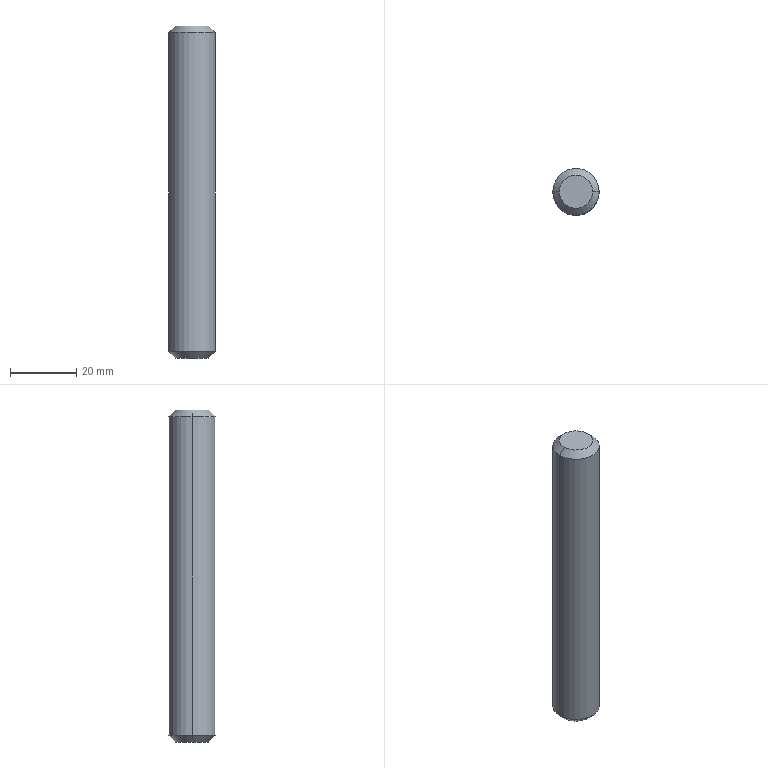Part | STEP file | CHOT 14X100 | 1 solid | 8 faces | box 14 x 14 x 100 mm | volume 15235 mm3 | cone 4 | cylinder 2 | plane 2 | commonest cylinder face diameters 14 x2
STEP:
#1=CARTESIAN_POINT('',(0.,0.,0.));
#2=DIRECTION('',(0.,0.,1.));
#3=DIRECTION('',(1.,0.,0.));
#4=AXIS2_PLACEMENT_3D('',#1,#2,#3);
#5=CARTESIAN_POINT('',(7.,0.,2.));
#6=VERTEX_POINT('',#5);
#7=CARTESIAN_POINT('',(-7.,0.,2.));
#8=VERTEX_POINT('',#7);
#9=CARTESIAN_POINT('',(0.,0.,2.));
#10=DIRECTION('',(0.,0.,1.));
#11=DIRECTION('',(1.,0.,0.));
#12=AXIS2_PLACEMENT_3D('',#9,#10,#11);
#13=CIRCLE('',#12,7.);
#14=CARTESIAN_POINT('',(0.,0.,0.));
#15=DIRECTION('',(0.,0.,1.));
#16=DIRECTION('',(1.,0.,0.));
#17=AXIS2_PLACEMENT_3D('',#14,#15,#16);
#18=CYLINDRICAL_SURFACE('',#17,7.);
#19=CARTESIAN_POINT('',(0.,2.));
#20=DIRECTION('',(1.,0.));
#21=VECTOR('',#20,1.);
#22=LINE('',#19,#21);
#23=(GEOMETRIC_REPRESENTATION_CONTEXT(2)PARAMETRIC_REPRESENTATION_CONTEXT()REPRESENTATION_CONTEXT('',''));
#24=DEFINITIONAL_REPRESENTATION('',(#22),#23);
#25=PCURVE('',#18,#24);
#26=CARTESIAN_POINT('',(0.,0.,2.));
#27=DIRECTION('',(0.,0.,1.));
#28=DIRECTION('',(1.,0.,0.));
#29=AXIS2_PLACEMENT_3D('',#26,#27,#28);
#30=CONICAL_SURFACE('',#29,7.,0.7854);
#31=CARTESIAN_POINT('',(0.,0.));
#32=DIRECTION('',(1.,0.));
#33=VECTOR('',#32,1.);
#34=LINE('',#31,#33);
#35=(GEOMETRIC_REPRESENTATION_CONTEXT(2)PARAMETRIC_REPRESENTATION_CONTEXT()REPRESENTATION_CONTEXT('',''));
#36=DEFINITIONAL_REPRESENTATION('',(#34),#35);
#37=PCURVE('',#30,#36);
#38=SURFACE_CURVE('',#13,(#25,#37),.PCURVE_S1.);
#39=EDGE_CURVE('',#6,#8,#38,.T.);
#40=ORIENTED_EDGE('',*,*,#39,.T.);
#41=CARTESIAN_POINT('',(-7.,0.,98.));
#42=VERTEX_POINT('',#41);
#43=CARTESIAN_POINT('',(-7.,0.,0.));
#44=DIRECTION('',(0.,0.,1.));
#45=VECTOR('',#44,1.);
#46=LINE('',#43,#45);
#47=CARTESIAN_POINT('',(3.142,0.));
#48=DIRECTION('',(0.,1.));
#49=VECTOR('',#48,1.);
#50=LINE('',#47,#49);
#51=(GEOMETRIC_REPRESENTATION_CONTEXT(2)PARAMETRIC_REPRESENTATION_CONTEXT()REPRESENTATION_CONTEXT('',''));
#52=DEFINITIONAL_REPRESENTATION('',(#50),#51);
#53=PCURVE('',#18,#52);
#54=CARTESIAN_POINT('',(0.,0.,0.));
#55=DIRECTION('',(0.,0.,1.));
#56=DIRECTION('',(1.,0.,0.));
#57=AXIS2_PLACEMENT_3D('',#54,#55,#56);
#58=CYLINDRICAL_SURFACE('',#57,7.);
#59=CARTESIAN_POINT('',(3.142,0.));
#60=DIRECTION('',(0.,1.));
#61=VECTOR('',#60,1.);
#62=LINE('',#59,#61);
#63=(GEOMETRIC_REPRESENTATION_CONTEXT(2)PARAMETRIC_REPRESENTATION_CONTEXT()REPRESENTATION_CONTEXT('',''));
#64=DEFINITIONAL_REPRESENTATION('',(#62),#63);
#65=PCURVE('',#58,#64);
#66=SURFACE_CURVE('',#46,(#53,#65),.PCURVE_S1.);
#67=EDGE_CURVE('',#8,#42,#66,.T.);
#68=ORIENTED_EDGE('',*,*,#67,.T.);
#69=CARTESIAN_POINT('',(7.,0.,98.));
#70=VERTEX_POINT('',#69);
#71=CARTESIAN_POINT('',(0.,0.,98.));
#72=DIRECTION('',(0.,0.,-1.));
#73=DIRECTION('',(1.,0.,0.));
#74=AXIS2_PLACEMENT_3D('',#71,#72,#73);
#75=CIRCLE('',#74,7.);
#76=CARTESIAN_POINT('',(6.283,98.));
#77=DIRECTION('',(-1.,0.));
#78=VECTOR('',#77,1.);
#79=LINE('',#76,#78);
#80=(GEOMETRIC_REPRESENTATION_CONTEXT(2)PARAMETRIC_REPRESENTATION_CONTEXT()REPRESENTATION_CONTEXT('',''));
#81=DEFINITIONAL_REPRESENTATION('',(#79),#80);
#82=PCURVE('',#18,#81);
#83=CARTESIAN_POINT('',(0.,0.,98.));
#84=DIRECTION('',(0.,0.,-1.));
#85=DIRECTION('',(-1.,0.,0.));
#86=AXIS2_PLACEMENT_3D('',#83,#84,#85);
#87=CONICAL_SURFACE('',#86,7.,0.7854);
#88=CARTESIAN_POINT('',(-3.142,0.));
#89=DIRECTION('',(1.,0.));
#90=VECTOR('',#89,1.);
#91=LINE('',#88,#90);
#92=(GEOMETRIC_REPRESENTATION_CONTEXT(2)PARAMETRIC_REPRESENTATION_CONTEXT()REPRESENTATION_CONTEXT('',''));
#93=DEFINITIONAL_REPRESENTATION('',(#91),#92);
#94=PCURVE('',#87,#93);
#95=SURFACE_CURVE('',#75,(#82,#94),.PCURVE_S1.);
#96=EDGE_CURVE('',#42,#70,#95,.T.);
#97=ORIENTED_EDGE('',*,*,#96,.T.);
#98=CARTESIAN_POINT('',(7.,0.,0.));
#99=DIRECTION('',(0.,0.,1.));
#100=VECTOR('',#99,1.);
#101=LINE('',#98,#100);
#102=CARTESIAN_POINT('',(0.,0.));
#103=DIRECTION('',(0.,1.));
#104=VECTOR('',#103,1.);
#105=LINE('',#102,#104);
#106=(GEOMETRIC_REPRESENTATION_CONTEXT(2)PARAMETRIC_REPRESENTATION_CONTEXT()REPRESENTATION_CONTEXT('',''));
#107=DEFINITIONAL_REPRESENTATION('',(#105),#106);
#108=PCURVE('',#18,#107);
#109=CARTESIAN_POINT('',(6.283,0.));
#110=DIRECTION('',(0.,1.));
#111=VECTOR('',#110,1.);
#112=LINE('',#109,#111);
#113=(GEOMETRIC_REPRESENTATION_CONTEXT(2)PARAMETRIC_REPRESENTATION_CONTEXT()REPRESENTATION_CONTEXT('',''));
#114=DEFINITIONAL_REPRESENTATION('',(#112),#113);
#115=PCURVE('',#58,#114);
#116=SURFACE_CURVE('',#101,(#108,#115),.PCURVE_S1.);
#117=EDGE_CURVE('',#6,#70,#116,.T.);
#118=ORIENTED_EDGE('',*,*,#117,.F.);
#119=EDGE_LOOP('',(#40,#68,#97,#118));
#120=FACE_BOUND('',#119,.T.);
#121=ADVANCED_FACE('',(#120),#18,.T.);
#122=CARTESIAN_POINT('',(5.,0.,-0.000000001));
#123=VERTEX_POINT('',#122);
#124=CARTESIAN_POINT('',(-5.,0.,-0.000000001));
#125=VERTEX_POINT('',#124);
#126=CARTESIAN_POINT('',(0.,0.,-0.000000001));
#127=DIRECTION('',(0.,0.,1.));
#128=DIRECTION('',(1.,0.,0.));
#129=AXIS2_PLACEMENT_3D('',#126,#127,#128);
#130=CIRCLE('',#129,5.);
#131=CARTESIAN_POINT('',(0.,-2.));
#132=DIRECTION('',(1.,0.));
#133=VECTOR('',#132,1.);
#134=LINE('',#131,#133);
#135=(GEOMETRIC_REPRESENTATION_CONTEXT(2)PARAMETRIC_REPRESENTATION_CONTEXT()REPRESENTATION_CONTEXT('',''));
#136=DEFINITIONAL_REPRESENTATION('',(#134),#135);
#137=PCURVE('',#30,#136);
#138=CARTESIAN_POINT('',(0.,0.,0.));
#139=DIRECTION('',(0.,0.,-1.));
#140=DIRECTION('',(-1.,0.,0.));
#141=AXIS2_PLACEMENT_3D('',#138,#139,#140);
#142=PLANE('',#141);
#143=CARTESIAN_POINT('',(-5.,0.));
#144=CARTESIAN_POINT('',(-5.,8.66));
#145=CARTESIAN_POINT('',(2.5,4.33));
#146=CARTESIAN_POINT('',(10.,0.));
#147=CARTESIAN_POINT('',(2.5,-4.33));
#148=CARTESIAN_POINT('',(-5.,-8.66));
#149=CARTESIAN_POINT('',(-5.,0.));
#150=(BOUNDED_CURVE()B_SPLINE_CURVE(2,(#143,#144,#145,#146,#147,#148,#149),.UNSPECIFIED.,.T.,.F.)B_SPLINE_CURVE_WITH_KNOTS((1,2,2,2,2,1),(-2.094,0.,2.094,4.189,6.283,8.378),.UNSPECIFIED.)CURVE()GEOMETRIC_REPRESENTATION_ITEM()RATIONAL_B_SPLINE_CURVE((1.,0.5,1.,0.5,1.,0.5,1.))REPRESENTATION_ITEM(''));
#151=(GEOMETRIC_REPRESENTATION_CONTEXT(2)PARAMETRIC_REPRESENTATION_CONTEXT()REPRESENTATION_CONTEXT('',''));
#152=DEFINITIONAL_REPRESENTATION('',(#150),#151);
#153=PCURVE('',#142,#152);
#154=SURFACE_CURVE('',#130,(#137,#153),.PCURVE_S1.);
#155=EDGE_CURVE('',#123,#125,#154,.T.);
#156=ORIENTED_EDGE('',*,*,#155,.T.);
#157=CARTESIAN_POINT('',(-7.,0.,2.));
#158=DIRECTION('',(-0.7071,0.,0.7071));
#159=VECTOR('',#158,1.);
#160=LINE('',#157,#159);
#161=CARTESIAN_POINT('',(3.142,0.));
#162=DIRECTION('',(0.,1.));
#163=VECTOR('',#162,1.);
#164=LINE('',#161,#163);
#165=(GEOMETRIC_REPRESENTATION_CONTEXT(2)PARAMETRIC_REPRESENTATION_CONTEXT()REPRESENTATION_CONTEXT('',''));
#166=DEFINITIONAL_REPRESENTATION('',(#164),#165);
#167=PCURVE('',#30,#166);
#168=CARTESIAN_POINT('',(0.,0.,2.));
#169=DIRECTION('',(0.,0.,1.));
#170=DIRECTION('',(1.,0.,0.));
#171=AXIS2_PLACEMENT_3D('',#168,#169,#170);
#172=CONICAL_SURFACE('',#171,7.,0.7854);
#173=CARTESIAN_POINT('',(3.142,0.));
#174=DIRECTION('',(0.,1.));
#175=VECTOR('',#174,1.);
#176=LINE('',#173,#175);
#177=(GEOMETRIC_REPRESENTATION_CONTEXT(2)PARAMETRIC_REPRESENTATION_CONTEXT()REPRESENTATION_CONTEXT('',''));
#178=DEFINITIONAL_REPRESENTATION('',(#176),#177);
#179=PCURVE('',#172,#178);
#180=SURFACE_CURVE('',#160,(#167,#179),.PCURVE_S1.);
#181=EDGE_CURVE('',#125,#8,#180,.T.);
#182=ORIENTED_EDGE('',*,*,#181,.T.);
#183=ORIENTED_EDGE('',*,*,#39,.F.);
#184=CARTESIAN_POINT('',(7.,0.,2.));
#185=DIRECTION('',(0.7071,0.,0.7071));
#186=VECTOR('',#185,1.);
#187=LINE('',#184,#186);
#188=CARTESIAN_POINT('',(0.,0.));
#189=DIRECTION('',(0.,1.));
#190=VECTOR('',#189,1.);
#191=LINE('',#188,#190);
#192=(GEOMETRIC_REPRESENTATION_CONTEXT(2)PARAMETRIC_REPRESENTATION_CONTEXT()REPRESENTATION_CONTEXT('',''));
#193=DEFINITIONAL_REPRESENTATION('',(#191),#192);
#194=PCURVE('',#30,#193);
#195=CARTESIAN_POINT('',(6.283,0.));
#196=DIRECTION('',(0.,1.));
#197=VECTOR('',#196,1.);
#198=LINE('',#195,#197);
#199=(GEOMETRIC_REPRESENTATION_CONTEXT(2)PARAMETRIC_REPRESENTATION_CONTEXT()REPRESENTATION_CONTEXT('',''));
#200=DEFINITIONAL_REPRESENTATION('',(#198),#199);
#201=PCURVE('',#172,#200);
#202=SURFACE_CURVE('',#187,(#194,#201),.PCURVE_S1.);
#203=EDGE_CURVE('',#123,#6,#202,.T.);
#204=ORIENTED_EDGE('',*,*,#203,.F.);
#205=EDGE_LOOP('',(#156,#182,#183,#204));
#206=FACE_BOUND('',#205,.T.);
#207=ADVANCED_FACE('',(#206),#30,.T.);
#208=CARTESIAN_POINT('',(-5.,0.,100.));
#209=VERTEX_POINT('',#208);
#210=CARTESIAN_POINT('',(5.,0.,100.));
#211=VERTEX_POINT('',#210);
#212=CARTESIAN_POINT('',(0.,0.,100.));
#213=DIRECTION('',(0.,0.,-1.));
#214=DIRECTION('',(-1.,0.,0.));
#215=AXIS2_PLACEMENT_3D('',#212,#213,#214);
#216=CIRCLE('',#215,5.);
#217=CARTESIAN_POINT('',(0.,-2.));
#218=DIRECTION('',(1.,0.));
#219=VECTOR('',#218,1.);
#220=LINE('',#217,#219);
#221=(GEOMETRIC_REPRESENTATION_CONTEXT(2)PARAMETRIC_REPRESENTATION_CONTEXT()REPRESENTATION_CONTEXT('',''));
#222=DEFINITIONAL_REPRESENTATION('',(#220),#221);
#223=PCURVE('',#87,#222);
#224=CARTESIAN_POINT('',(0.,0.,100.));
#225=DIRECTION('',(0.,0.,-1.));
#226=DIRECTION('',(-1.,0.,0.));
#227=AXIS2_PLACEMENT_3D('',#224,#225,#226);
#228=PLANE('',#227);
#229=CARTESIAN_POINT('',(0.,0.));
#230=DIRECTION('',(1.,0.));
#231=AXIS2_PLACEMENT_2D('',#229,#230);
#232=CIRCLE('',#231,5.);
#233=(GEOMETRIC_REPRESENTATION_CONTEXT(2)PARAMETRIC_REPRESENTATION_CONTEXT()REPRESENTATION_CONTEXT('',''));
#234=DEFINITIONAL_REPRESENTATION('',(#232),#233);
#235=PCURVE('',#228,#234);
#236=SURFACE_CURVE('',#216,(#223,#235),.PCURVE_S1.);
#237=EDGE_CURVE('',#209,#211,#236,.T.);
#238=ORIENTED_EDGE('',*,*,#237,.T.);
#239=CARTESIAN_POINT('',(7.,0.,98.));
#240=DIRECTION('',(0.7071,0.,-0.7071));
#241=VECTOR('',#240,1.);
#242=LINE('',#239,#241);
#243=CARTESIAN_POINT('',(3.142,0.));
#244=DIRECTION('',(0.,1.));
#245=VECTOR('',#244,1.);
#246=LINE('',#243,#245);
#247=(GEOMETRIC_REPRESENTATION_CONTEXT(2)PARAMETRIC_REPRESENTATION_CONTEXT()REPRESENTATION_CONTEXT('',''));
#248=DEFINITIONAL_REPRESENTATION('',(#246),#247);
#249=PCURVE('',#87,#248);
#250=CARTESIAN_POINT('',(0.,0.,98.));
#251=DIRECTION('',(0.,0.,-1.));
#252=DIRECTION('',(-1.,0.,0.));
#253=AXIS2_PLACEMENT_3D('',#250,#251,#252);
#254=CONICAL_SURFACE('',#253,7.,0.7854);
#255=CARTESIAN_POINT('',(3.142,0.));
#256=DIRECTION('',(0.,1.));
#257=VECTOR('',#256,1.);
#258=LINE('',#255,#257);
#259=(GEOMETRIC_REPRESENTATION_CONTEXT(2)PARAMETRIC_REPRESENTATION_CONTEXT()REPRESENTATION_CONTEXT('',''));
#260=DEFINITIONAL_REPRESENTATION('',(#258),#259);
#261=PCURVE('',#254,#260);
#262=SURFACE_CURVE('',#242,(#249,#261),.PCURVE_S1.);
#263=EDGE_CURVE('',#211,#70,#262,.T.);
#264=ORIENTED_EDGE('',*,*,#263,.T.);
#265=ORIENTED_EDGE('',*,*,#96,.F.);
#266=CARTESIAN_POINT('',(-7.,0.,98.));
#267=DIRECTION('',(-0.7071,0.,-0.7071));
#268=VECTOR('',#267,1.);
#269=LINE('',#266,#268);
#270=CARTESIAN_POINT('',(0.,0.));
#271=DIRECTION('',(0.,1.));
#272=VECTOR('',#271,1.);
#273=LINE('',#270,#272);
#274=(GEOMETRIC_REPRESENTATION_CONTEXT(2)PARAMETRIC_REPRESENTATION_CONTEXT()REPRESENTATION_CONTEXT('',''));
#275=DEFINITIONAL_REPRESENTATION('',(#273),#274);
#276=PCURVE('',#87,#275);
#277=CARTESIAN_POINT('',(6.283,0.));
#278=DIRECTION('',(0.,1.));
#279=VECTOR('',#278,1.);
#280=LINE('',#277,#279);
#281=(GEOMETRIC_REPRESENTATION_CONTEXT(2)PARAMETRIC_REPRESENTATION_CONTEXT()REPRESENTATION_CONTEXT('',''));
#282=DEFINITIONAL_REPRESENTATION('',(#280),#281);
#283=PCURVE('',#254,#282);
#284=SURFACE_CURVE('',#269,(#276,#283),.PCURVE_S1.);
#285=EDGE_CURVE('',#209,#42,#284,.T.);
#286=ORIENTED_EDGE('',*,*,#285,.F.);
#287=EDGE_LOOP('',(#238,#264,#265,#286));
#288=FACE_BOUND('',#287,.T.);
#289=ADVANCED_FACE('',(#288),#87,.T.);
#290=ORIENTED_EDGE('',*,*,#67,.F.);
#291=CARTESIAN_POINT('',(0.,0.,2.));
#292=DIRECTION('',(0.,0.,1.));
#293=DIRECTION('',(1.,0.,0.));
#294=AXIS2_PLACEMENT_3D('',#291,#292,#293);
#295=CIRCLE('',#294,7.);
#296=CARTESIAN_POINT('',(0.,2.));
#297=DIRECTION('',(1.,0.));
#298=VECTOR('',#297,1.);
#299=LINE('',#296,#298);
#300=(GEOMETRIC_REPRESENTATION_CONTEXT(2)PARAMETRIC_REPRESENTATION_CONTEXT()REPRESENTATION_CONTEXT('',''));
#301=DEFINITIONAL_REPRESENTATION('',(#299),#300);
#302=PCURVE('',#58,#301);
#303=CARTESIAN_POINT('',(0.,0.));
#304=DIRECTION('',(1.,0.));
#305=VECTOR('',#304,1.);
#306=LINE('',#303,#305);
#307=(GEOMETRIC_REPRESENTATION_CONTEXT(2)PARAMETRIC_REPRESENTATION_CONTEXT()REPRESENTATION_CONTEXT('',''));
#308=DEFINITIONAL_REPRESENTATION('',(#306),#307);
#309=PCURVE('',#172,#308);
#310=SURFACE_CURVE('',#295,(#302,#309),.PCURVE_S1.);
#311=EDGE_CURVE('',#8,#6,#310,.T.);
#312=ORIENTED_EDGE('',*,*,#311,.T.);
#313=ORIENTED_EDGE('',*,*,#117,.T.);
#314=CARTESIAN_POINT('',(0.,0.,98.));
#315=DIRECTION('',(0.,0.,-1.));
#316=DIRECTION('',(1.,0.,0.));
#317=AXIS2_PLACEMENT_3D('',#314,#315,#316);
#318=CIRCLE('',#317,7.);
#319=CARTESIAN_POINT('',(6.283,98.));
#320=DIRECTION('',(-1.,0.));
#321=VECTOR('',#320,1.);
#322=LINE('',#319,#321);
#323=(GEOMETRIC_REPRESENTATION_CONTEXT(2)PARAMETRIC_REPRESENTATION_CONTEXT()REPRESENTATION_CONTEXT('',''));
#324=DEFINITIONAL_REPRESENTATION('',(#322),#323);
#325=PCURVE('',#58,#324);
#326=CARTESIAN_POINT('',(3.142,0.));
#327=DIRECTION('',(1.,0.));
#328=VECTOR('',#327,1.);
#329=LINE('',#326,#328);
#330=(GEOMETRIC_REPRESENTATION_CONTEXT(2)PARAMETRIC_REPRESENTATION_CONTEXT()REPRESENTATION_CONTEXT('',''));
#331=DEFINITIONAL_REPRESENTATION('',(#329),#330);
#332=PCURVE('',#254,#331);
#333=SURFACE_CURVE('',#318,(#325,#332),.PCURVE_S1.);
#334=EDGE_CURVE('',#70,#42,#333,.T.);
#335=ORIENTED_EDGE('',*,*,#334,.T.);
#336=EDGE_LOOP('',(#290,#312,#313,#335));
#337=FACE_BOUND('',#336,.T.);
#338=ADVANCED_FACE('',(#337),#58,.T.);
#339=ORIENTED_EDGE('',*,*,#181,.F.);
#340=CARTESIAN_POINT('',(0.,0.,-0.000000001));
#341=DIRECTION('',(0.,0.,1.));
#342=DIRECTION('',(1.,0.,0.));
#343=AXIS2_PLACEMENT_3D('',#340,#341,#342);
#344=CIRCLE('',#343,5.);
#345=CARTESIAN_POINT('',(0.,-2.));
#346=DIRECTION('',(1.,0.));
#347=VECTOR('',#346,1.);
#348=LINE('',#345,#347);
#349=(GEOMETRIC_REPRESENTATION_CONTEXT(2)PARAMETRIC_REPRESENTATION_CONTEXT()REPRESENTATION_CONTEXT('',''));
#350=DEFINITIONAL_REPRESENTATION('',(#348),#349);
#351=PCURVE('',#172,#350);
#352=CARTESIAN_POINT('',(-5.,0.));
#353=CARTESIAN_POINT('',(-5.,8.66));
#354=CARTESIAN_POINT('',(2.5,4.33));
#355=CARTESIAN_POINT('',(10.,0.));
#356=CARTESIAN_POINT('',(2.5,-4.33));
#357=CARTESIAN_POINT('',(-5.,-8.66));
#358=CARTESIAN_POINT('',(-5.,0.));
#359=(BOUNDED_CURVE()B_SPLINE_CURVE(2,(#352,#353,#354,#355,#356,#357,#358),.UNSPECIFIED.,.T.,.F.)B_SPLINE_CURVE_WITH_KNOTS((1,2,2,2,2,1),(-2.094,0.,2.094,4.189,6.283,8.378),.UNSPECIFIED.)CURVE()GEOMETRIC_REPRESENTATION_ITEM()RATIONAL_B_SPLINE_CURVE((1.,0.5,1.,0.5,1.,0.5,1.))REPRESENTATION_ITEM(''));
#360=(GEOMETRIC_REPRESENTATION_CONTEXT(2)PARAMETRIC_REPRESENTATION_CONTEXT()REPRESENTATION_CONTEXT('',''));
#361=DEFINITIONAL_REPRESENTATION('',(#359),#360);
#362=PCURVE('',#142,#361);
#363=SURFACE_CURVE('',#344,(#351,#362),.PCURVE_S1.);
#364=EDGE_CURVE('',#125,#123,#363,.T.);
#365=ORIENTED_EDGE('',*,*,#364,.T.);
#366=ORIENTED_EDGE('',*,*,#203,.T.);
#367=ORIENTED_EDGE('',*,*,#311,.F.);
#368=EDGE_LOOP('',(#339,#365,#366,#367));
#369=FACE_BOUND('',#368,.T.);
#370=ADVANCED_FACE('',(#369),#172,.T.);
#371=ORIENTED_EDGE('',*,*,#263,.F.);
#372=CARTESIAN_POINT('',(0.,0.,100.));
#373=DIRECTION('',(0.,0.,-1.));
#374=DIRECTION('',(-1.,0.,0.));
#375=AXIS2_PLACEMENT_3D('',#372,#373,#374);
#376=CIRCLE('',#375,5.);
#377=CARTESIAN_POINT('',(0.,-2.));
#378=DIRECTION('',(1.,0.));
#379=VECTOR('',#378,1.);
#380=LINE('',#377,#379);
#381=(GEOMETRIC_REPRESENTATION_CONTEXT(2)PARAMETRIC_REPRESENTATION_CONTEXT()REPRESENTATION_CONTEXT('',''));
#382=DEFINITIONAL_REPRESENTATION('',(#380),#381);
#383=PCURVE('',#254,#382);
#384=CARTESIAN_POINT('',(0.,0.));
#385=DIRECTION('',(1.,0.));
#386=AXIS2_PLACEMENT_2D('',#384,#385);
#387=CIRCLE('',#386,5.);
#388=(GEOMETRIC_REPRESENTATION_CONTEXT(2)PARAMETRIC_REPRESENTATION_CONTEXT()REPRESENTATION_CONTEXT('',''));
#389=DEFINITIONAL_REPRESENTATION('',(#387),#388);
#390=PCURVE('',#228,#389);
#391=SURFACE_CURVE('',#376,(#383,#390),.PCURVE_S1.);
#392=EDGE_CURVE('',#211,#209,#391,.T.);
#393=ORIENTED_EDGE('',*,*,#392,.T.);
#394=ORIENTED_EDGE('',*,*,#285,.T.);
#395=ORIENTED_EDGE('',*,*,#334,.F.);
#396=EDGE_LOOP('',(#371,#393,#394,#395));
#397=FACE_BOUND('',#396,.T.);
#398=ADVANCED_FACE('',(#397),#254,.T.);
#399=ORIENTED_EDGE('',*,*,#155,.F.);
#400=ORIENTED_EDGE('',*,*,#364,.F.);
#401=EDGE_LOOP('',(#399,#400));
#402=FACE_BOUND('',#401,.T.);
#403=ADVANCED_FACE('',(#402),#142,.T.);
#404=ORIENTED_EDGE('',*,*,#237,.F.);
#405=ORIENTED_EDGE('',*,*,#392,.F.);
#406=EDGE_LOOP('',(#404,#405));
#407=FACE_BOUND('',#406,.T.);
#408=ADVANCED_FACE('',(#407),#228,.F.);
#409=CLOSED_SHELL('',(#121,#207,#289,#338,#370,#398,#403,#408));
#410=MANIFOLD_SOLID_BREP('',#409);
#411=(LENGTH_UNIT()NAMED_UNIT(*)SI_UNIT(.MILLI.,.METRE.));
#412=UNCERTAINTY_MEASURE_WITH_UNIT(LENGTH_MEASURE(0.0000001),#411,'','');
#413=(NAMED_UNIT(*)PLANE_ANGLE_UNIT()SI_UNIT($,.RADIAN.));
#414=(NAMED_UNIT(*)SI_UNIT($,.STERADIAN.)SOLID_ANGLE_UNIT());
#415=(GEOMETRIC_REPRESENTATION_CONTEXT(3)GLOBAL_UNCERTAINTY_ASSIGNED_CONTEXT((#412))GLOBAL_UNIT_ASSIGNED_CONTEXT((#411,#413,#414))REPRESENTATION_CONTEXT('',''));
#416=ADVANCED_BREP_SHAPE_REPRESENTATION('',(#4,#410),#415);